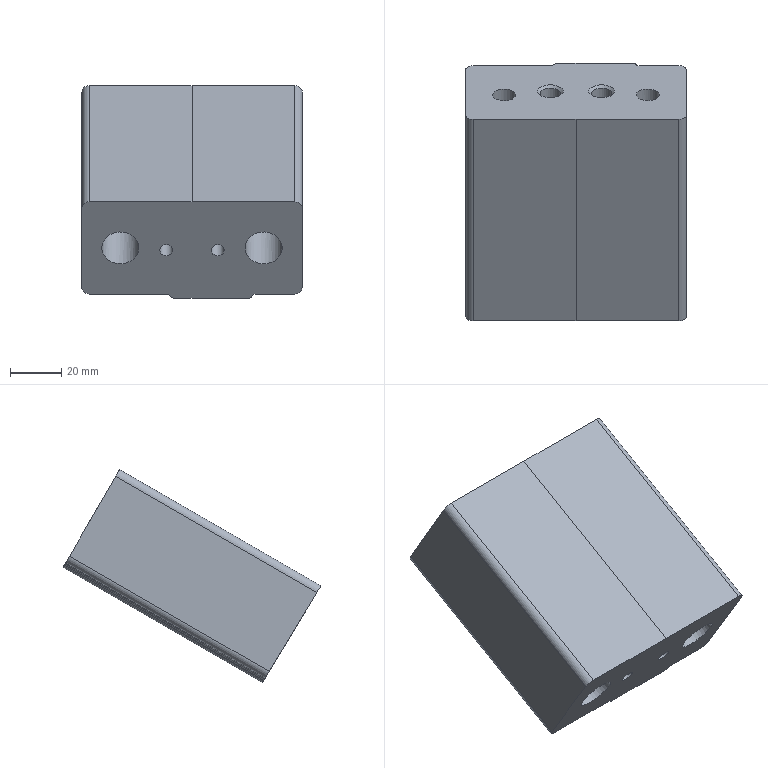Part | NX | features solid 2 | 1 solid | 32 faces | box 86.008 x 100.559 x 83.036 mm | volume 306507 mm3 | plane 13 | spline 9 | cylinder 8 | cone 2 | commonest cylinder face diameters 5.1 x2 8 x2 9.007 x2 14.508 x2
STEP:
#1=CARTESIAN_POINT('',(-139.757,107.914,-0.2414));
#2=VERTEX_POINT('',#1);
#3=CARTESIAN_POINT('',(-137.826,107.52,0.4097));
#4=CARTESIAN_POINT('',(-139.728,108.056,-0.4768));
#5=CARTESIAN_POINT('',(-141.803,107.738,0.04954));
#6=CARTESIAN_POINT('',(-142.834,106.756,1.674));
#7=CARTESIAN_POINT('',(-142.223,105.683,3.45));
#8=CARTESIAN_POINT('',(-140.322,105.148,4.335));
#9=CARTESIAN_POINT('',(-138.25,105.464,3.811));
#10=CARTESIAN_POINT('',(-137.215,106.447,2.186));
#11=CARTESIAN_POINT('',(-137.826,107.52,0.4097));
#12=CARTESIAN_POINT('',(-139.728,108.056,-0.4768));
#13=CARTESIAN_POINT('',(-141.803,107.738,0.04954));
#14=B_SPLINE_CURVE_WITH_KNOTS('',3,(#3,#4,#5,#6,#7,#8,#9,#10,#11,#12,#13),.UNSPECIFIED.,.T.,.F.,(1,1,1,1,1,1,1,1,1,1,1,1,1,1,1),(-0.005979,-0.003986,-0.001993,0.,0.001993,0.003986,0.005979,0.007972,0.009965,0.01196,0.01395,0.01594,0.01794,0.01993,0.02192),.UNSPECIFIED.);
#15=EDGE_CURVE('',#2,#2,#14,.T.);
#16=ORIENTED_EDGE('',*,*,#15,.T.);
#17=EDGE_LOOP('',(#16));
#18=FACE_BOUND('',#17,.T.);
#19=CARTESIAN_POINT('',(-170.771,106.072,2.807));
#20=VERTEX_POINT('',#19);
#21=CARTESIAN_POINT('',(-172.347,109.015,-2.062));
#22=CARTESIAN_POINT('',(-169.984,106.071,2.808));
#23=CARTESIAN_POINT('',(-172.341,103.131,7.673));
#24=CARTESIAN_POINT('',(-178.016,101.913,9.689));
#25=CARTESIAN_POINT('',(-183.705,103.128,7.681));
#26=CARTESIAN_POINT('',(-186.063,106.069,2.815));
#27=CARTESIAN_POINT('',(-183.717,109.007,-2.046));
#28=CARTESIAN_POINT('',(-178.037,110.229,-4.07));
#29=CARTESIAN_POINT('',(-172.347,109.015,-2.062));
#30=CARTESIAN_POINT('',(-169.984,106.071,2.808));
#31=CARTESIAN_POINT('',(-172.341,103.131,7.673));
#32=B_SPLINE_CURVE_WITH_KNOTS('',3,(#21,#22,#23,#24,#25,#26,#27,#28,#29,#30,#31),.UNSPECIFIED.,.T.,.F.,(1,1,1,1,1,1,1,1,1,1,1,1,1,1,1),(-0.01701,-0.01134,-0.005669,0.,0.005669,0.01134,0.01701,0.02268,0.02835,0.03402,0.03968,0.04535,0.05102,0.05669,0.06236),.UNSPECIFIED.);
#33=EDGE_CURVE('',#20,#20,#32,.T.);
#34=ORIENTED_EDGE('',*,*,#33,.F.);
#35=EDGE_LOOP('',(#34));
#36=FACE_BOUND('',#35,.T.);
#37=CARTESIAN_POINT('',(-129.279,106.076,2.8));
#38=VERTEX_POINT('',#37);
#39=CARTESIAN_POINT('',(-127.705,103.133,7.67));
#40=CARTESIAN_POINT('',(-130.066,106.077,2.798));
#41=CARTESIAN_POINT('',(-127.707,109.017,-2.066));
#42=CARTESIAN_POINT('',(-122.031,110.234,-4.079));
#43=CARTESIAN_POINT('',(-116.343,109.02,-2.068));
#44=CARTESIAN_POINT('',(-113.987,106.078,2.8));
#45=CARTESIAN_POINT('',(-116.335,103.141,7.659));
#46=CARTESIAN_POINT('',(-122.016,101.919,9.68));
#47=CARTESIAN_POINT('',(-127.705,103.133,7.67));
#48=CARTESIAN_POINT('',(-130.066,106.077,2.798));
#49=CARTESIAN_POINT('',(-127.707,109.017,-2.066));
#50=B_SPLINE_CURVE_WITH_KNOTS('',3,(#39,#40,#41,#42,#43,#44,#45,#46,#47,#48,#49),.UNSPECIFIED.,.T.,.F.,(1,1,1,1,1,1,1,1,1,1,1,1,1,1,1),(-0.01701,-0.01134,-0.005669,0.,0.005669,0.01134,0.01701,0.02268,0.02835,0.03402,0.03968,0.04535,0.05102,0.05669,0.06236),.UNSPECIFIED.);
#51=EDGE_CURVE('',#38,#38,#50,.T.);
#52=ORIENTED_EDGE('',*,*,#51,.F.);
#53=EDGE_LOOP('',(#52));
#54=FACE_BOUND('',#53,.T.);
#55=CARTESIAN_POINT('',(-110.021,95.216,20.774));
#56=VERTEX_POINT('',#55);
#57=CARTESIAN_POINT('',(-107.021,96.769,18.206));
#58=VERTEX_POINT('',#57);
#59=CARTESIAN_POINT('',(-110.021,95.216,20.774));
#60=CARTESIAN_POINT('',(-109.229,95.216,20.774));
#61=CARTESIAN_POINT('',(-107.676,95.554,20.216));
#62=CARTESIAN_POINT('',(-107.021,96.359,18.885));
#63=CARTESIAN_POINT('',(-107.021,96.769,18.206));
#64=B_SPLINE_CURVE_WITH_KNOTS('',3,(#59,#60,#61,#62,#63),.UNSPECIFIED.,.F.,.F.,(4,1,4),(0.,0.002343,0.004687),.UNSPECIFIED.);
#65=EDGE_CURVE('',#56,#58,#64,.T.);
#66=ORIENTED_EDGE('',*,*,#65,.F.);
#67=CARTESIAN_POINT('',(-150.023,95.214,20.773));
#68=VERTEX_POINT('',#67);
#69=CARTESIAN_POINT('',(-150.023,95.214,20.773));
#70=CARTESIAN_POINT('',(-136.689,95.213,20.773));
#71=CARTESIAN_POINT('',(-123.355,95.214,20.773));
#72=CARTESIAN_POINT('',(-110.021,95.216,20.774));
#73=B_SPLINE_CURVE_WITH_KNOTS('',3,(#69,#70,#71,#72),.UNSPECIFIED.,.F.,.F.,(4,4),(0.,0.04),.UNSPECIFIED.);
#74=EDGE_CURVE('',#68,#56,#73,.T.);
#75=ORIENTED_EDGE('',*,*,#74,.F.);
#76=CARTESIAN_POINT('',(-190.021,95.216,20.774));
#77=VERTEX_POINT('',#76);
#78=CARTESIAN_POINT('',(-190.021,95.216,20.774));
#79=CARTESIAN_POINT('',(-176.688,95.215,20.773));
#80=CARTESIAN_POINT('',(-163.356,95.214,20.773));
#81=CARTESIAN_POINT('',(-150.023,95.214,20.773));
#82=B_SPLINE_CURVE_WITH_KNOTS('',3,(#78,#79,#80,#81),.UNSPECIFIED.,.F.,.F.,(4,4),(0.,0.04),.UNSPECIFIED.);
#83=EDGE_CURVE('',#77,#68,#82,.T.);
#84=ORIENTED_EDGE('',*,*,#83,.F.);
#85=CARTESIAN_POINT('',(-193.021,96.768,18.208));
#86=VERTEX_POINT('',#85);
#87=CARTESIAN_POINT('',(-193.021,96.768,18.208));
#88=CARTESIAN_POINT('',(-193.021,96.358,18.886));
#89=CARTESIAN_POINT('',(-192.369,95.555,20.214));
#90=CARTESIAN_POINT('',(-190.813,95.216,20.774));
#91=CARTESIAN_POINT('',(-190.021,95.216,20.774));
#92=B_SPLINE_CURVE_WITH_KNOTS('',3,(#87,#88,#89,#90,#91),.UNSPECIFIED.,.F.,.F.,(4,1,4),(0.,0.002342,0.004684),.UNSPECIFIED.);
#93=EDGE_CURVE('',#86,#77,#92,.T.);
#94=ORIENTED_EDGE('',*,*,#93,.F.);
#95=CARTESIAN_POINT('',(-193.029,115.406,-12.632));
#96=VERTEX_POINT('',#95);
#97=CARTESIAN_POINT('',(-193.029,115.406,-12.632));
#98=CARTESIAN_POINT('',(-193.026,109.193,-2.352));
#99=CARTESIAN_POINT('',(-193.024,102.98,7.927));
#100=CARTESIAN_POINT('',(-193.021,96.768,18.208));
#101=B_SPLINE_CURVE_WITH_KNOTS('',3,(#97,#98,#99,#100),.UNSPECIFIED.,.F.,.F.,(4,4),(0.,0.03603),.UNSPECIFIED.);
#102=EDGE_CURVE('',#96,#86,#101,.T.);
#103=ORIENTED_EDGE('',*,*,#102,.F.);
#104=CARTESIAN_POINT('',(-190.029,116.958,-15.2));
#105=VERTEX_POINT('',#104);
#106=CARTESIAN_POINT('',(-190.029,116.958,-15.2));
#107=CARTESIAN_POINT('',(-190.821,116.958,-15.2));
#108=CARTESIAN_POINT('',(-192.374,116.621,-14.642));
#109=CARTESIAN_POINT('',(-193.029,115.816,-13.31));
#110=CARTESIAN_POINT('',(-193.029,115.406,-12.632));
#111=B_SPLINE_CURVE_WITH_KNOTS('',3,(#106,#107,#108,#109,#110),.UNSPECIFIED.,.F.,.F.,(4,1,4),(0.,0.002343,0.004687),.UNSPECIFIED.);
#112=EDGE_CURVE('',#105,#96,#111,.T.);
#113=ORIENTED_EDGE('',*,*,#112,.F.);
#114=CARTESIAN_POINT('',(-160.273,116.956,-15.202));
#115=VERTEX_POINT('',#114);
#116=CARTESIAN_POINT('',(-160.273,116.956,-15.202));
#117=CARTESIAN_POINT('',(-170.192,116.956,-15.202));
#118=CARTESIAN_POINT('',(-180.11,116.957,-15.201));
#119=CARTESIAN_POINT('',(-190.029,116.958,-15.2));
#120=B_SPLINE_CURVE_WITH_KNOTS('',3,(#116,#117,#118,#119),.UNSPECIFIED.,.F.,.F.,(4,4),(0.,0.02976),.UNSPECIFIED.);
#121=EDGE_CURVE('',#115,#105,#120,.T.);
#122=ORIENTED_EDGE('',*,*,#121,.F.);
#123=CARTESIAN_POINT('',(-158.541,117.473,-16.058));
#124=VERTEX_POINT('',#123);
#125=CARTESIAN_POINT('',(-158.541,117.473,-16.058));
#126=CARTESIAN_POINT('',(-158.893,117.158,-15.536));
#127=CARTESIAN_POINT('',(-159.57,116.956,-15.202));
#128=CARTESIAN_POINT('',(-160.273,116.956,-15.202));
#129=B_SPLINE_CURVE_WITH_KNOTS('',3,(#125,#126,#127,#128),.UNSPECIFIED.,.F.,.F.,(4,4),(0.,0.002093),.UNSPECIFIED.);
#130=EDGE_CURVE('',#124,#115,#129,.T.);
#131=ORIENTED_EDGE('',*,*,#130,.F.);
#132=CARTESIAN_POINT('',(-156.809,117.99,-16.913));
#133=VERTEX_POINT('',#132);
#134=CARTESIAN_POINT('',(-156.809,117.99,-16.913));
#135=CARTESIAN_POINT('',(-157.513,117.99,-16.913));
#136=CARTESIAN_POINT('',(-158.19,117.788,-16.579));
#137=CARTESIAN_POINT('',(-158.541,117.473,-16.058));
#138=B_SPLINE_CURVE_WITH_KNOTS('',3,(#134,#135,#136,#137),.UNSPECIFIED.,.F.,.F.,(4,4),(0.,0.002093),.UNSPECIFIED.);
#139=EDGE_CURVE('',#133,#124,#138,.T.);
#140=ORIENTED_EDGE('',*,*,#139,.F.);
#141=CARTESIAN_POINT('',(-150.023,117.99,-16.914));
#142=VERTEX_POINT('',#141);
#143=CARTESIAN_POINT('',(-150.023,117.99,-16.914));
#144=CARTESIAN_POINT('',(-152.285,117.99,-16.914));
#145=CARTESIAN_POINT('',(-154.547,117.99,-16.914));
#146=CARTESIAN_POINT('',(-156.809,117.99,-16.913));
#147=B_SPLINE_CURVE_WITH_KNOTS('',3,(#143,#144,#145,#146),.UNSPECIFIED.,.F.,.F.,(4,4),(0.,0.006786),.UNSPECIFIED.);
#148=EDGE_CURVE('',#142,#133,#147,.T.);
#149=ORIENTED_EDGE('',*,*,#148,.F.);
#150=CARTESIAN_POINT('',(-128.427,117.991,-16.913));
#151=VERTEX_POINT('',#150);
#152=CARTESIAN_POINT('',(-128.427,117.991,-16.913));
#153=CARTESIAN_POINT('',(-135.626,117.99,-16.913));
#154=CARTESIAN_POINT('',(-142.825,117.99,-16.914));
#155=CARTESIAN_POINT('',(-150.023,117.99,-16.914));
#156=B_SPLINE_CURVE_WITH_KNOTS('',3,(#152,#153,#154,#155),.UNSPECIFIED.,.F.,.F.,(4,4),(0.,0.0216),.UNSPECIFIED.);
#157=EDGE_CURVE('',#151,#142,#156,.T.);
#158=ORIENTED_EDGE('',*,*,#157,.F.);
#159=CARTESIAN_POINT('',(-126.695,117.474,-16.057));
#160=VERTEX_POINT('',#159);
#161=CARTESIAN_POINT('',(-126.695,117.474,-16.057));
#162=CARTESIAN_POINT('',(-127.047,117.789,-16.579));
#163=CARTESIAN_POINT('',(-127.724,117.991,-16.913));
#164=CARTESIAN_POINT('',(-128.427,117.991,-16.913));
#165=B_SPLINE_CURVE_WITH_KNOTS('',3,(#161,#162,#163,#164),.UNSPECIFIED.,.F.,.F.,(4,4),(0.,0.002093),.UNSPECIFIED.);
#166=EDGE_CURVE('',#160,#151,#165,.T.);
#167=ORIENTED_EDGE('',*,*,#166,.F.);
#168=CARTESIAN_POINT('',(-124.963,116.956,-15.201));
#169=VERTEX_POINT('',#168);
#170=CARTESIAN_POINT('',(-124.963,116.956,-15.201));
#171=CARTESIAN_POINT('',(-125.667,116.956,-15.201));
#172=CARTESIAN_POINT('',(-126.343,117.159,-15.536));
#173=CARTESIAN_POINT('',(-126.695,117.474,-16.057));
#174=B_SPLINE_CURVE_WITH_KNOTS('',3,(#170,#171,#172,#173),.UNSPECIFIED.,.F.,.F.,(4,4),(0.,0.002093),.UNSPECIFIED.);
#175=EDGE_CURVE('',#169,#160,#174,.T.);
#176=ORIENTED_EDGE('',*,*,#175,.F.);
#177=CARTESIAN_POINT('',(-110.029,116.958,-15.2));
#178=VERTEX_POINT('',#177);
#179=CARTESIAN_POINT('',(-110.029,116.958,-15.2));
#180=CARTESIAN_POINT('',(-115.007,116.957,-15.201));
#181=CARTESIAN_POINT('',(-119.985,116.957,-15.201));
#182=CARTESIAN_POINT('',(-124.963,116.956,-15.201));
#183=B_SPLINE_CURVE_WITH_KNOTS('',3,(#179,#180,#181,#182),.UNSPECIFIED.,.F.,.F.,(4,4),(0.,0.01493),.UNSPECIFIED.);
#184=EDGE_CURVE('',#178,#169,#183,.T.);
#185=ORIENTED_EDGE('',*,*,#184,.F.);
#186=CARTESIAN_POINT('',(-107.029,115.407,-12.633));
#187=VERTEX_POINT('',#186);
#188=CARTESIAN_POINT('',(-107.029,115.407,-12.633));
#189=CARTESIAN_POINT('',(-107.029,115.817,-13.311));
#190=CARTESIAN_POINT('',(-107.681,116.62,-14.64));
#191=CARTESIAN_POINT('',(-109.237,116.958,-15.2));
#192=CARTESIAN_POINT('',(-110.029,116.958,-15.2));
#193=B_SPLINE_CURVE_WITH_KNOTS('',3,(#188,#189,#190,#191,#192),.UNSPECIFIED.,.F.,.F.,(4,1,4),(0.,0.002343,0.004686),.UNSPECIFIED.);
#194=EDGE_CURVE('',#187,#178,#193,.T.);
#195=ORIENTED_EDGE('',*,*,#194,.F.);
#196=CARTESIAN_POINT('',(-107.021,96.769,18.206));
#197=CARTESIAN_POINT('',(-107.024,102.981,7.926));
#198=CARTESIAN_POINT('',(-107.026,109.194,-2.354));
#199=CARTESIAN_POINT('',(-107.029,115.407,-12.633));
#200=B_SPLINE_CURVE_WITH_KNOTS('',3,(#196,#197,#198,#199),.UNSPECIFIED.,.F.,.F.,(4,4),(0.,0.03603),.UNSPECIFIED.);
#201=EDGE_CURVE('',#58,#187,#200,.T.);
#202=ORIENTED_EDGE('',*,*,#201,.F.);
#203=EDGE_LOOP('',(#66,#75,#84,#94,#103,#113,#122,#131,#140,#149,#158,#167,#176,#185,#195,#202));
#204=FACE_BOUND('',#203,.T.);
#205=CARTESIAN_POINT('',(-159.757,107.914,-0.2413));
#206=VERTEX_POINT('',#205);
#207=CARTESIAN_POINT('',(-157.826,107.52,0.4098));
#208=CARTESIAN_POINT('',(-159.728,108.056,-0.4768));
#209=CARTESIAN_POINT('',(-161.803,107.738,0.0497));
#210=CARTESIAN_POINT('',(-162.834,106.756,1.674));
#211=CARTESIAN_POINT('',(-162.223,105.683,3.45));
#212=CARTESIAN_POINT('',(-160.322,105.148,4.335));
#213=CARTESIAN_POINT('',(-158.25,105.464,3.811));
#214=CARTESIAN_POINT('',(-157.215,106.447,2.186));
#215=CARTESIAN_POINT('',(-157.826,107.52,0.4098));
#216=CARTESIAN_POINT('',(-159.728,108.056,-0.4768));
#217=CARTESIAN_POINT('',(-161.803,107.738,0.0497));
#218=B_SPLINE_CURVE_WITH_KNOTS('',3,(#207,#208,#209,#210,#211,#212,#213,#214,#215,#216,#217),.UNSPECIFIED.,.T.,.F.,(1,1,1,1,1,1,1,1,1,1,1,1,1,1,1),(-0.005979,-0.003986,-0.001993,0.,0.001993,0.003986,0.005979,0.007972,0.009965,0.01196,0.01395,0.01594,0.01794,0.01993,0.02192),.UNSPECIFIED.);
#219=EDGE_CURVE('',#206,#206,#218,.T.);
#220=ORIENTED_EDGE('',*,*,#219,.T.);
#221=EDGE_LOOP('',(#220));
#222=FACE_BOUND('',#221,.T.);
#223=CARTESIAN_POINT('',(-193.54,95.075,21.009));
#224=CARTESIAN_POINT('',(-193.54,95.31,20.621));
#225=CARTESIAN_POINT('',(-193.542,102.949,7.979));
#226=CARTESIAN_POINT('',(-193.544,110.589,-4.661));
#227=CARTESIAN_POINT('',(-193.545,117.994,-16.913));
#228=CARTESIAN_POINT('',(-164.528,95.073,21.004));
#229=CARTESIAN_POINT('',(-164.528,95.308,20.615));
#230=CARTESIAN_POINT('',(-164.53,102.947,7.974));
#231=CARTESIAN_POINT('',(-164.532,110.587,-4.666));
#232=CARTESIAN_POINT('',(-164.534,117.992,-16.918));
#233=CARTESIAN_POINT('',(-135.516,95.074,21.));
#234=CARTESIAN_POINT('',(-135.517,95.309,20.612));
#235=CARTESIAN_POINT('',(-135.518,102.948,7.971));
#236=CARTESIAN_POINT('',(-135.52,110.588,-4.67));
#237=CARTESIAN_POINT('',(-135.522,117.993,-16.922));
#238=CARTESIAN_POINT('',(-106.505,95.08,21.));
#239=CARTESIAN_POINT('',(-106.505,95.315,20.612));
#240=CARTESIAN_POINT('',(-106.506,102.954,7.971));
#241=CARTESIAN_POINT('',(-106.508,110.594,-4.67));
#242=CARTESIAN_POINT('',(-106.51,117.999,-16.922));
#243=B_SPLINE_SURFACE_WITH_KNOTS('',3,3,((#223,#224,#225,#226,#227),(#228,#229,#230,#231,#232),(#233,#234,#235,#236,#237),(#238,#239,#240,#241,#242)),.UNSPECIFIED.,.F.,.F.,.F.,(4,4),(4,1,4),(0.02905,0.971),(-0.03172,0.,1.),.UNSPECIFIED.);
#244=ADVANCED_FACE('',(#18,#36,#54,#204,#222),#243,.F.);
#245=CARTESIAN_POINT('',(-107.029,193.273,32.325));
#246=VERTEX_POINT('',#245);
#247=CARTESIAN_POINT('',(-107.029,159.412,12.774));
#248=DIRECTION('',(0.000000832,0.866,0.5));
#249=VECTOR('',#248,1000.);
#250=LINE('',#247,#249);
#251=EDGE_CURVE('',#246,#187,#250,.F.);
#252=ORIENTED_EDGE('',*,*,#251,.T.);
#253=ORIENTED_EDGE('',*,*,#194,.T.);
#254=CARTESIAN_POINT('',(-110.029,194.773,29.728));
#255=VERTEX_POINT('',#254);
#256=CARTESIAN_POINT('',(-110.029,160.911,10.177));
#257=DIRECTION('',(0.000000832,0.866,0.5));
#258=VECTOR('',#257,1000.);
#259=LINE('',#256,#258);
#260=EDGE_CURVE('',#255,#178,#259,.F.);
#261=ORIENTED_EDGE('',*,*,#260,.F.);
#262=CARTESIAN_POINT('',(-107.029,193.273,32.325));
#263=CARTESIAN_POINT('',(-107.029,193.669,31.639));
#264=CARTESIAN_POINT('',(-107.681,194.445,30.294));
#265=CARTESIAN_POINT('',(-109.237,194.773,29.728));
#266=CARTESIAN_POINT('',(-110.029,194.773,29.728));
#267=B_SPLINE_CURVE_WITH_KNOTS('',3,(#262,#263,#264,#265,#266),.UNSPECIFIED.,.F.,.F.,(4,1,4),(0.,0.002343,0.004685),.UNSPECIFIED.);
#268=EDGE_CURVE('',#246,#255,#267,.T.);
#269=ORIENTED_EDGE('',*,*,#268,.F.);
#270=EDGE_LOOP('',(#252,#253,#261,#269));
#271=FACE_BOUND('',#270,.T.);
#272=CARTESIAN_POINT('',(-107.029,114.94,-12.903));
#273=CARTESIAN_POINT('',(-107.029,193.273,32.325));
#274=CARTESIAN_POINT('',(-107.029,115.332,-13.582));
#275=CARTESIAN_POINT('',(-107.029,193.666,31.645));
#276=CARTESIAN_POINT('',(-107.679,116.115,-14.939));
#277=CARTESIAN_POINT('',(-107.679,194.449,30.289));
#278=CARTESIAN_POINT('',(-109.247,116.439,-15.5));
#279=CARTESIAN_POINT('',(-109.247,194.773,29.728));
#280=CARTESIAN_POINT('',(-110.029,116.439,-15.5));
#281=CARTESIAN_POINT('',(-110.029,194.773,29.728));
#282=B_SPLINE_SURFACE_WITH_KNOTS('',3,1,((#272,#273),(#274,#275),(#276,#277),(#278,#279),(#280,#281)),.SURF_OF_LINEAR_EXTRUSION.,.F.,.F.,.F.,(4,1,4),(2,2),(0.,0.5,1.),(0.,1.),.UNSPECIFIED.);
#283=ADVANCED_FACE('',(#271),#282,.T.);
#284=ORIENTED_EDGE('',*,*,#260,.T.);
#285=ORIENTED_EDGE('',*,*,#184,.T.);
#286=CARTESIAN_POINT('',(-124.963,194.773,29.728));
#287=VERTEX_POINT('',#286);
#288=CARTESIAN_POINT('',(-124.963,160.911,10.177));
#289=DIRECTION('',(0.000000832,0.866,0.5));
#290=VECTOR('',#289,1000.);
#291=LINE('',#288,#290);
#292=EDGE_CURVE('',#287,#169,#291,.F.);
#293=ORIENTED_EDGE('',*,*,#292,.F.);
#294=CARTESIAN_POINT('',(-150.099,194.773,29.728));
#295=DIRECTION('',(1.,-0.000001199,0.000000412));
#296=VECTOR('',#295,1000.);
#297=LINE('',#294,#296);
#298=EDGE_CURVE('',#255,#287,#297,.F.);
#299=ORIENTED_EDGE('',*,*,#298,.F.);
#300=EDGE_LOOP('',(#284,#285,#293,#299));
#301=FACE_BOUND('',#300,.T.);
#302=CARTESIAN_POINT('',(-110.029,160.911,10.177));
#303=DIRECTION('',(0.000000956,0.5,-0.866));
#304=DIRECTION('',(-1.,0.000001199,-0.000000412));
#305=AXIS2_PLACEMENT_3D('',#302,#303,#304);
#306=PLANE('',#305);
#307=ADVANCED_FACE('',(#301),#306,.T.);
#308=ORIENTED_EDGE('',*,*,#292,.T.);
#309=ORIENTED_EDGE('',*,*,#175,.T.);
#310=CARTESIAN_POINT('',(-126.695,195.273,28.862));
#311=VERTEX_POINT('',#310);
#312=CARTESIAN_POINT('',(-126.695,161.411,9.311));
#313=DIRECTION('',(0.000000832,0.866,0.5));
#314=VECTOR('',#313,1000.);
#315=LINE('',#312,#314);
#316=EDGE_CURVE('',#311,#160,#315,.F.);
#317=ORIENTED_EDGE('',*,*,#316,.F.);
#318=CARTESIAN_POINT('',(-124.963,194.773,29.728));
#319=CARTESIAN_POINT('',(-125.666,194.773,29.728));
#320=CARTESIAN_POINT('',(-126.343,194.968,29.389));
#321=CARTESIAN_POINT('',(-126.695,195.273,28.862));
#322=B_SPLINE_CURVE_WITH_KNOTS('',3,(#318,#319,#320,#321),.UNSPECIFIED.,.F.,.F.,(4,4),(0.,0.002093),.UNSPECIFIED.);
#323=EDGE_CURVE('',#287,#311,#322,.T.);
#324=ORIENTED_EDGE('',*,*,#323,.F.);
#325=EDGE_LOOP('',(#308,#309,#317,#324));
#326=FACE_BOUND('',#325,.T.);
#327=CARTESIAN_POINT('',(-124.963,116.49,-15.471));
#328=CARTESIAN_POINT('',(-124.963,194.773,29.728));
#329=CARTESIAN_POINT('',(-125.661,116.49,-15.471));
#330=CARTESIAN_POINT('',(-125.661,194.773,29.728));
#331=CARTESIAN_POINT('',(-126.347,116.688,-15.815));
#332=CARTESIAN_POINT('',(-126.347,194.971,29.384));
#333=CARTESIAN_POINT('',(-126.695,116.989,-16.337));
#334=CARTESIAN_POINT('',(-126.695,195.273,28.862));
#335=B_SPLINE_SURFACE_WITH_KNOTS('',3,1,((#327,#328),(#329,#330),(#331,#332),(#333,#334)),.SURF_OF_LINEAR_EXTRUSION.,.F.,.F.,.F.,(4,4),(2,2),(0.,1.),(0.,1.),.PIECEWISE_BEZIER_KNOTS.);
#336=ADVANCED_FACE('',(#326),#335,.T.);
#337=ORIENTED_EDGE('',*,*,#316,.T.);
#338=ORIENTED_EDGE('',*,*,#166,.T.);
#339=CARTESIAN_POINT('',(-128.427,195.773,27.996));
#340=VERTEX_POINT('',#339);
#341=CARTESIAN_POINT('',(-128.427,161.911,8.445));
#342=DIRECTION('',(0.000000832,0.866,0.5));
#343=VECTOR('',#342,1000.);
#344=LINE('',#341,#343);
#345=EDGE_CURVE('',#340,#151,#344,.F.);
#346=ORIENTED_EDGE('',*,*,#345,.F.);
#347=CARTESIAN_POINT('',(-126.695,195.273,28.862));
#348=CARTESIAN_POINT('',(-127.047,195.577,28.334));
#349=CARTESIAN_POINT('',(-127.724,195.773,27.996));
#350=CARTESIAN_POINT('',(-128.427,195.773,27.996));
#351=B_SPLINE_CURVE_WITH_KNOTS('',3,(#347,#348,#349,#350),.UNSPECIFIED.,.F.,.F.,(4,4),(0.,0.002093),.UNSPECIFIED.);
#352=EDGE_CURVE('',#311,#340,#351,.T.);
#353=ORIENTED_EDGE('',*,*,#352,.F.);
#354=EDGE_LOOP('',(#337,#338,#346,#353));
#355=FACE_BOUND('',#354,.T.);
#356=CARTESIAN_POINT('',(-126.695,117.007,-16.327));
#357=CARTESIAN_POINT('',(-126.695,195.273,28.862));
#358=CARTESIAN_POINT('',(-127.044,117.309,-16.85));
#359=CARTESIAN_POINT('',(-127.044,195.575,28.339));
#360=CARTESIAN_POINT('',(-127.731,117.507,-17.193));
#361=CARTESIAN_POINT('',(-127.731,195.773,27.996));
#362=CARTESIAN_POINT('',(-128.427,117.507,-17.193));
#363=CARTESIAN_POINT('',(-128.427,195.773,27.996));
#364=B_SPLINE_SURFACE_WITH_KNOTS('',3,1,((#356,#357),(#358,#359),(#360,#361),(#362,#363)),.SURF_OF_LINEAR_EXTRUSION.,.F.,.F.,.F.,(4,4),(2,2),(0.,1.),(0.,1.),.PIECEWISE_BEZIER_KNOTS.);
#365=ADVANCED_FACE('',(#355),#364,.T.);
#366=ORIENTED_EDGE('',*,*,#345,.T.);
#367=ORIENTED_EDGE('',*,*,#157,.T.);
#368=CARTESIAN_POINT('',(-150.023,195.773,27.996));
#369=VERTEX_POINT('',#368);
#370=CARTESIAN_POINT('',(-150.023,161.911,8.445));
#371=DIRECTION('',(0.000000832,0.866,0.5));
#372=VECTOR('',#371,1000.);
#373=LINE('',#370,#372);
#374=EDGE_CURVE('',#369,#142,#373,.F.);
#375=ORIENTED_EDGE('',*,*,#374,.F.);
#376=CARTESIAN_POINT('',(-150.099,195.773,27.996));
#377=DIRECTION('',(1.,-0.000001199,0.000000412));
#378=VECTOR('',#377,1000.);
#379=LINE('',#376,#378);
#380=EDGE_CURVE('',#340,#369,#379,.F.);
#381=ORIENTED_EDGE('',*,*,#380,.F.);
#382=EDGE_LOOP('',(#366,#367,#375,#381));
#383=FACE_BOUND('',#382,.T.);
#384=CARTESIAN_POINT('',(-128.427,161.911,8.445));
#385=DIRECTION('',(0.000000956,0.5,-0.866));
#386=DIRECTION('',(-1.,0.000001199,-0.000000412));
#387=AXIS2_PLACEMENT_3D('',#384,#385,#386);
#388=PLANE('',#387);
#389=ADVANCED_FACE('',(#383),#388,.T.);
#390=ORIENTED_EDGE('',*,*,#374,.T.);
#391=ORIENTED_EDGE('',*,*,#148,.T.);
#392=CARTESIAN_POINT('',(-156.809,195.773,27.996));
#393=VERTEX_POINT('',#392);
#394=CARTESIAN_POINT('',(-156.809,161.911,8.445));
#395=DIRECTION('',(0.000000832,0.866,0.5));
#396=VECTOR('',#395,1000.);
#397=LINE('',#394,#396);
#398=EDGE_CURVE('',#393,#133,#397,.F.);
#399=ORIENTED_EDGE('',*,*,#398,.F.);
#400=CARTESIAN_POINT('',(-150.099,195.773,27.996));
#401=DIRECTION('',(1.,0.000001199,-0.000003741));
#402=VECTOR('',#401,1000.);
#403=LINE('',#400,#402);
#404=EDGE_CURVE('',#369,#393,#403,.F.);
#405=ORIENTED_EDGE('',*,*,#404,.F.);
#406=EDGE_LOOP('',(#390,#391,#399,#405));
#407=FACE_BOUND('',#406,.T.);
#408=CARTESIAN_POINT('',(-150.023,161.911,8.445));
#409=DIRECTION('',(-0.000003839,0.5,-0.866));
#410=DIRECTION('',(-1.,-0.000001199,0.000003741));
#411=AXIS2_PLACEMENT_3D('',#408,#409,#410);
#412=PLANE('',#411);
#413=ADVANCED_FACE('',(#407),#412,.T.);
#414=ORIENTED_EDGE('',*,*,#398,.T.);
#415=ORIENTED_EDGE('',*,*,#139,.T.);
#416=CARTESIAN_POINT('',(-158.541,195.273,28.862));
#417=VERTEX_POINT('',#416);
#418=CARTESIAN_POINT('',(-158.541,161.411,9.311));
#419=DIRECTION('',(0.000000832,0.866,0.5));
#420=VECTOR('',#419,1000.);
#421=LINE('',#418,#420);
#422=EDGE_CURVE('',#417,#124,#421,.F.);
#423=ORIENTED_EDGE('',*,*,#422,.F.);
#424=CARTESIAN_POINT('',(-156.809,195.773,27.996));
#425=CARTESIAN_POINT('',(-157.513,195.773,27.996));
#426=CARTESIAN_POINT('',(-158.19,195.577,28.334));
#427=CARTESIAN_POINT('',(-158.541,195.273,28.862));
#428=B_SPLINE_CURVE_WITH_KNOTS('',3,(#424,#425,#426,#427),.UNSPECIFIED.,.F.,.F.,(4,4),(0.,0.002093),.UNSPECIFIED.);
#429=EDGE_CURVE('',#393,#417,#428,.T.);
#430=ORIENTED_EDGE('',*,*,#429,.F.);
#431=EDGE_LOOP('',(#414,#415,#423,#430));
#432=FACE_BOUND('',#431,.T.);
#433=CARTESIAN_POINT('',(-156.809,117.506,-17.193));
#434=CARTESIAN_POINT('',(-156.809,195.773,27.996));
#435=CARTESIAN_POINT('',(-157.507,117.506,-17.193));
#436=CARTESIAN_POINT('',(-157.507,195.773,27.996));
#437=CARTESIAN_POINT('',(-158.193,117.307,-16.849));
#438=CARTESIAN_POINT('',(-158.193,195.574,28.34));
#439=CARTESIAN_POINT('',(-158.541,117.006,-16.327));
#440=CARTESIAN_POINT('',(-158.541,195.273,28.862));
#441=B_SPLINE_SURFACE_WITH_KNOTS('',3,1,((#433,#434),(#435,#436),(#437,#438),(#439,#440)),.SURF_OF_LINEAR_EXTRUSION.,.F.,.F.,.F.,(4,4),(2,2),(0.,1.),(0.,1.),.PIECEWISE_BEZIER_KNOTS.);
#442=ADVANCED_FACE('',(#432),#441,.T.);
#443=ORIENTED_EDGE('',*,*,#422,.T.);
#444=ORIENTED_EDGE('',*,*,#130,.T.);
#445=CARTESIAN_POINT('',(-160.273,194.773,29.728));
#446=VERTEX_POINT('',#445);
#447=CARTESIAN_POINT('',(-160.273,160.911,10.177));
#448=DIRECTION('',(0.000000832,0.866,0.5));
#449=VECTOR('',#448,1000.);
#450=LINE('',#447,#449);
#451=EDGE_CURVE('',#446,#115,#450,.F.);
#452=ORIENTED_EDGE('',*,*,#451,.F.);
#453=CARTESIAN_POINT('',(-158.541,195.273,28.862));
#454=CARTESIAN_POINT('',(-158.893,194.968,29.389));
#455=CARTESIAN_POINT('',(-159.57,194.773,29.728));
#456=CARTESIAN_POINT('',(-160.273,194.773,29.728));
#457=B_SPLINE_CURVE_WITH_KNOTS('',3,(#453,#454,#455,#456),.UNSPECIFIED.,.F.,.F.,(4,4),(0.,0.002093),.UNSPECIFIED.);
#458=EDGE_CURVE('',#417,#446,#457,.T.);
#459=ORIENTED_EDGE('',*,*,#458,.F.);
#460=EDGE_LOOP('',(#443,#444,#452,#459));
#461=FACE_BOUND('',#460,.T.);
#462=CARTESIAN_POINT('',(-158.541,116.989,-16.337));
#463=CARTESIAN_POINT('',(-158.541,195.273,28.862));
#464=CARTESIAN_POINT('',(-158.89,116.687,-15.814));
#465=CARTESIAN_POINT('',(-158.89,194.971,29.385));
#466=CARTESIAN_POINT('',(-159.578,116.489,-15.471));
#467=CARTESIAN_POINT('',(-159.578,194.773,29.728));
#468=CARTESIAN_POINT('',(-160.273,116.489,-15.471));
#469=CARTESIAN_POINT('',(-160.273,194.773,29.728));
#470=B_SPLINE_SURFACE_WITH_KNOTS('',3,1,((#462,#463),(#464,#465),(#466,#467),(#468,#469)),.SURF_OF_LINEAR_EXTRUSION.,.F.,.F.,.F.,(4,4),(2,2),(0.,1.),(0.,1.),.PIECEWISE_BEZIER_KNOTS.);
#471=ADVANCED_FACE('',(#461),#470,.T.);
#472=ORIENTED_EDGE('',*,*,#451,.T.);
#473=ORIENTED_EDGE('',*,*,#121,.T.);
#474=CARTESIAN_POINT('',(-190.029,194.773,29.728));
#475=VERTEX_POINT('',#474);
#476=CARTESIAN_POINT('',(-190.029,160.911,10.177));
#477=DIRECTION('',(0.000000832,0.866,0.5));
#478=VECTOR('',#477,1000.);
#479=LINE('',#476,#478);
#480=EDGE_CURVE('',#475,#105,#479,.F.);
#481=ORIENTED_EDGE('',*,*,#480,.F.);
#482=CARTESIAN_POINT('',(-150.099,194.773,29.728));
#483=DIRECTION('',(1.,0.000001199,-0.000003741));
#484=VECTOR('',#483,1000.);
#485=LINE('',#482,#484);
#486=EDGE_CURVE('',#446,#475,#485,.F.);
#487=ORIENTED_EDGE('',*,*,#486,.F.);
#488=EDGE_LOOP('',(#472,#473,#481,#487));
#489=FACE_BOUND('',#488,.T.);
#490=CARTESIAN_POINT('',(-160.273,160.911,10.177));
#491=DIRECTION('',(-0.000003839,0.5,-0.866));
#492=DIRECTION('',(-1.,-0.000001199,0.000003741));
#493=AXIS2_PLACEMENT_3D('',#490,#491,#492);
#494=PLANE('',#493);
#495=ADVANCED_FACE('',(#489),#494,.T.);
#496=ORIENTED_EDGE('',*,*,#480,.T.);
#497=ORIENTED_EDGE('',*,*,#112,.T.);
#498=CARTESIAN_POINT('',(-193.029,193.273,32.326));
#499=VERTEX_POINT('',#498);
#500=CARTESIAN_POINT('',(-193.029,159.411,12.775));
#501=DIRECTION('',(0.000000832,0.866,0.5));
#502=VECTOR('',#501,1000.);
#503=LINE('',#500,#502);
#504=EDGE_CURVE('',#499,#96,#503,.F.);
#505=ORIENTED_EDGE('',*,*,#504,.F.);
#506=CARTESIAN_POINT('',(-190.029,194.773,29.728));
#507=CARTESIAN_POINT('',(-190.821,194.773,29.728));
#508=CARTESIAN_POINT('',(-192.374,194.447,30.292));
#509=CARTESIAN_POINT('',(-193.029,193.669,31.64));
#510=CARTESIAN_POINT('',(-193.029,193.273,32.326));
#511=B_SPLINE_CURVE_WITH_KNOTS('',3,(#506,#507,#508,#509,#510),.UNSPECIFIED.,.F.,.F.,(4,1,4),(0.,0.002343,0.004686),.UNSPECIFIED.);
#512=EDGE_CURVE('',#475,#499,#511,.T.);
#513=ORIENTED_EDGE('',*,*,#512,.F.);
#514=EDGE_LOOP('',(#496,#497,#505,#513));
#515=FACE_BOUND('',#514,.T.);
#516=CARTESIAN_POINT('',(-190.029,116.439,-15.5));
#517=CARTESIAN_POINT('',(-190.029,194.773,29.728));
#518=CARTESIAN_POINT('',(-190.814,116.439,-15.5));
#519=CARTESIAN_POINT('',(-190.814,194.773,29.728));
#520=CARTESIAN_POINT('',(-192.381,116.115,-14.937));
#521=CARTESIAN_POINT('',(-192.38,194.448,30.29));
#522=CARTESIAN_POINT('',(-193.029,115.33,-13.579));
#523=CARTESIAN_POINT('',(-193.029,193.664,31.649));
#524=CARTESIAN_POINT('',(-193.029,114.939,-12.902));
#525=CARTESIAN_POINT('',(-193.029,193.273,32.326));
#526=B_SPLINE_SURFACE_WITH_KNOTS('',3,1,((#516,#517),(#518,#519),(#520,#521),(#522,#523),(#524,#525)),.SURF_OF_LINEAR_EXTRUSION.,.F.,.F.,.F.,(4,1,4),(2,2),(0.,0.5,1.),(0.,1.),.UNSPECIFIED.);
#527=ADVANCED_FACE('',(#515),#526,.T.);
#528=ORIENTED_EDGE('',*,*,#504,.T.);
#529=ORIENTED_EDGE('',*,*,#102,.T.);
#530=CARTESIAN_POINT('',(-193.021,175.259,63.526));
#531=VERTEX_POINT('',#530);
#532=CARTESIAN_POINT('',(-193.021,141.397,43.975));
#533=DIRECTION('',(0.000000832,0.866,0.5));
#534=VECTOR('',#533,1000.);
#535=LINE('',#532,#534);
#536=EDGE_CURVE('',#531,#86,#535,.F.);
#537=ORIENTED_EDGE('',*,*,#536,.F.);
#538=CARTESIAN_POINT('',(-193.025,185.26,46.203));
#539=DIRECTION('',(-0.0002148,0.5,-0.866));
#540=VECTOR('',#539,1000.);
#541=LINE('',#538,#540);
#542=EDGE_CURVE('',#499,#531,#541,.F.);
#543=ORIENTED_EDGE('',*,*,#542,.F.);
#544=EDGE_LOOP('',(#528,#529,#537,#543));
#545=FACE_BOUND('',#544,.T.);
#546=CARTESIAN_POINT('',(-193.029,159.411,12.775));
#547=DIRECTION('',(-1.,-0.0001067,0.0001864));
#548=DIRECTION('',(0.0002148,-0.5,0.866));
#549=AXIS2_PLACEMENT_3D('',#546,#547,#548);
#550=PLANE('',#549);
#551=ADVANCED_FACE('',(#545),#550,.T.);
#552=ORIENTED_EDGE('',*,*,#536,.T.);
#553=ORIENTED_EDGE('',*,*,#93,.T.);
#554=CARTESIAN_POINT('',(-190.021,173.759,66.123));
#555=VERTEX_POINT('',#554);
#556=CARTESIAN_POINT('',(-190.021,139.898,46.572));
#557=DIRECTION('',(0.000000832,0.866,0.5));
#558=VECTOR('',#557,1000.);
#559=LINE('',#556,#558);
#560=EDGE_CURVE('',#555,#77,#559,.F.);
#561=ORIENTED_EDGE('',*,*,#560,.F.);
#562=CARTESIAN_POINT('',(-193.021,175.259,63.526));
#563=CARTESIAN_POINT('',(-193.021,174.863,64.212));
#564=CARTESIAN_POINT('',(-192.368,174.086,65.556));
#565=CARTESIAN_POINT('',(-190.813,173.759,66.123));
#566=CARTESIAN_POINT('',(-190.021,173.759,66.123));
#567=B_SPLINE_CURVE_WITH_KNOTS('',3,(#562,#563,#564,#565,#566),.UNSPECIFIED.,.F.,.F.,(4,1,4),(0.,0.002342,0.004683),.UNSPECIFIED.);
#568=EDGE_CURVE('',#531,#555,#567,.T.);
#569=ORIENTED_EDGE('',*,*,#568,.F.);
#570=EDGE_LOOP('',(#552,#553,#561,#569));
#571=FACE_BOUND('',#570,.T.);
#572=CARTESIAN_POINT('',(-193.021,96.244,17.905));
#573=CARTESIAN_POINT('',(-193.021,175.259,63.526));
#574=CARTESIAN_POINT('',(-193.021,95.848,18.591));
#575=CARTESIAN_POINT('',(-193.021,174.863,64.212));
#576=CARTESIAN_POINT('',(-192.369,95.072,19.935));
#577=CARTESIAN_POINT('',(-192.368,174.086,65.556));
#578=CARTESIAN_POINT('',(-190.813,94.745,20.502));
#579=CARTESIAN_POINT('',(-190.813,173.759,66.123));
#580=CARTESIAN_POINT('',(-190.021,94.745,20.502));
#581=CARTESIAN_POINT('',(-190.021,173.759,66.123));
#582=B_SPLINE_SURFACE_WITH_KNOTS('',3,1,((#572,#573),(#574,#575),(#576,#577),(#578,#579),(#580,#581)),.SURF_OF_LINEAR_EXTRUSION.,.F.,.F.,.F.,(4,1,4),(2,2),(0.,0.5,1.),(0.,1.),.UNSPECIFIED.);
#583=ADVANCED_FACE('',(#571),#582,.T.);
#584=ORIENTED_EDGE('',*,*,#560,.T.);
#585=ORIENTED_EDGE('',*,*,#83,.T.);
#586=CARTESIAN_POINT('',(-150.023,173.759,66.123));
#587=VERTEX_POINT('',#586);
#588=CARTESIAN_POINT('',(-150.023,139.898,46.572));
#589=DIRECTION('',(0.000000832,0.866,0.5));
#590=VECTOR('',#589,1000.);
#591=LINE('',#588,#590);
#592=EDGE_CURVE('',#587,#68,#591,.F.);
#593=ORIENTED_EDGE('',*,*,#592,.F.);
#594=CARTESIAN_POINT('',(-150.099,173.759,66.123));
#595=DIRECTION('',(-1.,-0.000001199,0.000003741));
#596=VECTOR('',#595,1000.);
#597=LINE('',#594,#596);
#598=EDGE_CURVE('',#555,#587,#597,.F.);
#599=ORIENTED_EDGE('',*,*,#598,.F.);
#600=EDGE_LOOP('',(#584,#585,#593,#599));
#601=FACE_BOUND('',#600,.T.);
#602=CARTESIAN_POINT('',(-190.021,139.898,46.572));
#603=DIRECTION('',(0.000003839,-0.5,0.866));
#604=DIRECTION('',(1.,0.000001199,-0.000003741));
#605=AXIS2_PLACEMENT_3D('',#602,#603,#604);
#606=PLANE('',#605);
#607=ADVANCED_FACE('',(#601),#606,.T.);
#608=ORIENTED_EDGE('',*,*,#592,.T.);
#609=ORIENTED_EDGE('',*,*,#74,.T.);
#610=CARTESIAN_POINT('',(-110.021,173.759,66.123));
#611=VERTEX_POINT('',#610);
#612=CARTESIAN_POINT('',(-110.021,139.898,46.572));
#613=DIRECTION('',(0.000000832,0.866,0.5));
#614=VECTOR('',#613,1000.);
#615=LINE('',#612,#614);
#616=EDGE_CURVE('',#611,#56,#615,.F.);
#617=ORIENTED_EDGE('',*,*,#616,.F.);
#618=CARTESIAN_POINT('',(-150.099,173.759,66.123));
#619=DIRECTION('',(-1.,0.000001199,-0.000000412));
#620=VECTOR('',#619,1000.);
#621=LINE('',#618,#620);
#622=EDGE_CURVE('',#587,#611,#621,.F.);
#623=ORIENTED_EDGE('',*,*,#622,.F.);
#624=EDGE_LOOP('',(#608,#609,#617,#623));
#625=FACE_BOUND('',#624,.T.);
#626=CARTESIAN_POINT('',(-150.023,139.898,46.572));
#627=DIRECTION('',(-0.000000956,-0.5,0.866));
#628=DIRECTION('',(1.,-0.000001199,0.000000412));
#629=AXIS2_PLACEMENT_3D('',#626,#627,#628);
#630=PLANE('',#629);
#631=ADVANCED_FACE('',(#625),#630,.T.);
#632=ORIENTED_EDGE('',*,*,#616,.T.);
#633=ORIENTED_EDGE('',*,*,#65,.T.);
#634=CARTESIAN_POINT('',(-107.021,175.259,63.525));
#635=VERTEX_POINT('',#634);
#636=CARTESIAN_POINT('',(-107.021,141.398,43.974));
#637=DIRECTION('',(0.000000832,0.866,0.5));
#638=VECTOR('',#637,1000.);
#639=LINE('',#636,#638);
#640=EDGE_CURVE('',#635,#58,#639,.F.);
#641=ORIENTED_EDGE('',*,*,#640,.F.);
#642=CARTESIAN_POINT('',(-110.021,173.759,66.123));
#643=CARTESIAN_POINT('',(-109.229,173.759,66.123));
#644=CARTESIAN_POINT('',(-107.676,174.085,65.558));
#645=CARTESIAN_POINT('',(-107.021,174.863,64.211));
#646=CARTESIAN_POINT('',(-107.021,175.259,63.525));
#647=B_SPLINE_CURVE_WITH_KNOTS('',3,(#642,#643,#644,#645,#646),.UNSPECIFIED.,.F.,.F.,(4,1,4),(0.,0.002343,0.004686),.UNSPECIFIED.);
#648=EDGE_CURVE('',#611,#635,#647,.T.);
#649=ORIENTED_EDGE('',*,*,#648,.F.);
#650=EDGE_LOOP('',(#632,#633,#641,#649));
#651=FACE_BOUND('',#650,.T.);
#652=CARTESIAN_POINT('',(-110.021,94.745,20.502));
#653=CARTESIAN_POINT('',(-110.021,173.759,66.123));
#654=CARTESIAN_POINT('',(-109.236,94.745,20.502));
#655=CARTESIAN_POINT('',(-109.236,173.759,66.123));
#656=CARTESIAN_POINT('',(-107.669,95.07,19.94));
#657=CARTESIAN_POINT('',(-107.669,174.084,65.56));
#658=CARTESIAN_POINT('',(-107.021,95.854,18.581));
#659=CARTESIAN_POINT('',(-107.021,174.868,64.202));
#660=CARTESIAN_POINT('',(-107.021,96.245,17.904));
#661=CARTESIAN_POINT('',(-107.021,175.259,63.525));
#662=B_SPLINE_SURFACE_WITH_KNOTS('',3,1,((#652,#653),(#654,#655),(#656,#657),(#658,#659),(#660,#661)),.SURF_OF_LINEAR_EXTRUSION.,.F.,.F.,.F.,(4,1,4),(2,2),(0.,0.5,1.),(0.,1.),.UNSPECIFIED.);
#663=ADVANCED_FACE('',(#651),#662,.T.);
#664=CARTESIAN_POINT('',(-107.025,185.27,46.187));
#665=DIRECTION('',(0.0002148,-0.5,0.866));
#666=VECTOR('',#665,1000.);
#667=LINE('',#664,#666);
#668=EDGE_CURVE('',#635,#246,#667,.F.);
#669=ORIENTED_EDGE('',*,*,#668,.F.);
#670=ORIENTED_EDGE('',*,*,#640,.T.);
#671=ORIENTED_EDGE('',*,*,#201,.T.);
#672=ORIENTED_EDGE('',*,*,#251,.F.);
#673=EDGE_LOOP('',(#669,#670,#671,#672));
#674=FACE_BOUND('',#673,.T.);
#675=CARTESIAN_POINT('',(-107.021,141.398,43.974));
#676=DIRECTION('',(1.,0.0001067,-0.0001864));
#677=DIRECTION('',(-0.0002148,0.5,-0.866));
#678=AXIS2_PLACEMENT_3D('',#675,#676,#677);
#679=PLANE('',#678);
#680=ADVANCED_FACE('',(#674),#679,.T.);
#681=CARTESIAN_POINT('',(-140.025,187.266,42.729));
#682=VERTEX_POINT('',#681);
#683=CARTESIAN_POINT('',(-140.025,184.766,47.059));
#684=DIRECTION('',(-0.000000832,-0.866,-0.5));
#685=DIRECTION('',(0.,0.5,-0.866));
#686=AXIS2_PLACEMENT_3D('',#683,#684,#685);
#687=CIRCLE('',#686,5.);
#688=EDGE_CURVE('',#682,#682,#687,.T.);
#689=ORIENTED_EDGE('',*,*,#688,.T.);
#690=EDGE_LOOP('',(#689));
#691=FACE_BOUND('',#690,.T.);
#692=CARTESIAN_POINT('',(-160.025,187.266,42.729));
#693=VERTEX_POINT('',#692);
#694=CARTESIAN_POINT('',(-160.025,184.766,47.059));
#695=DIRECTION('',(-0.000000832,-0.866,-0.5));
#696=DIRECTION('',(0.,0.5,-0.866));
#697=AXIS2_PLACEMENT_3D('',#694,#695,#696);
#698=CIRCLE('',#697,5.);
#699=EDGE_CURVE('',#693,#693,#698,.T.);
#700=ORIENTED_EDGE('',*,*,#699,.T.);
#701=EDGE_LOOP('',(#700));
#702=FACE_BOUND('',#701,.T.);
#703=CARTESIAN_POINT('',(-178.024,181.096,53.415));
#704=VERTEX_POINT('',#703);
#705=CARTESIAN_POINT('',(-178.025,183.348,49.515));
#706=DIRECTION('',(-0.000000832,-0.866,-0.5));
#707=DIRECTION('',(0.0001031,-0.5,0.866));
#708=AXIS2_PLACEMENT_3D('',#705,#706,#707);
#709=ELLIPSE('',#708,4.504,4.503);
#710=EDGE_CURVE('',#704,#704,#709,.T.);
#711=ORIENTED_EDGE('',*,*,#710,.T.);
#712=EDGE_LOOP('',(#711));
#713=FACE_BOUND('',#712,.T.);
#714=CARTESIAN_POINT('',(-122.023,181.102,53.405));
#715=VERTEX_POINT('',#714);
#716=CARTESIAN_POINT('',(-122.024,183.354,49.504));
#717=DIRECTION('',(-0.000000832,-0.866,-0.5));
#718=DIRECTION('',(0.0003265,-0.5,0.866));
#719=AXIS2_PLACEMENT_3D('',#716,#717,#718);
#720=ELLIPSE('',#719,4.504,4.503);
#721=EDGE_CURVE('',#715,#715,#720,.T.);
#722=ORIENTED_EDGE('',*,*,#721,.T.);
#723=EDGE_LOOP('',(#722));
#724=FACE_BOUND('',#723,.T.);
#725=ORIENTED_EDGE('',*,*,#648,.T.);
#726=ORIENTED_EDGE('',*,*,#668,.T.);
#727=ORIENTED_EDGE('',*,*,#268,.T.);
#728=ORIENTED_EDGE('',*,*,#298,.T.);
#729=ORIENTED_EDGE('',*,*,#323,.T.);
#730=ORIENTED_EDGE('',*,*,#352,.T.);
#731=ORIENTED_EDGE('',*,*,#380,.T.);
#732=ORIENTED_EDGE('',*,*,#404,.T.);
#733=ORIENTED_EDGE('',*,*,#429,.T.);
#734=ORIENTED_EDGE('',*,*,#458,.T.);
#735=ORIENTED_EDGE('',*,*,#486,.T.);
#736=ORIENTED_EDGE('',*,*,#512,.T.);
#737=ORIENTED_EDGE('',*,*,#542,.T.);
#738=ORIENTED_EDGE('',*,*,#568,.T.);
#739=ORIENTED_EDGE('',*,*,#598,.T.);
#740=ORIENTED_EDGE('',*,*,#622,.T.);
#741=EDGE_LOOP('',(#725,#726,#727,#728,#729,#730,#731,#732,#733,#734,#735,#736,#737,#738,#739,#740));
#742=FACE_BOUND('',#741,.T.);
#743=CARTESIAN_POINT('',(-150.099,185.265,46.195));
#744=DIRECTION('',(-0.000000832,-0.866,-0.5));
#745=DIRECTION('',(0.000001441,-0.5,0.866));
#746=AXIS2_PLACEMENT_3D('',#743,#744,#745);
#747=PLANE('',#746);
#748=ADVANCED_FACE('',(#691,#702,#713,#724,#742),#747,.F.);
#749=CARTESIAN_POINT('',(-178.025,134.933,14.992));
#750=VERTEX_POINT('',#749);
#751=CARTESIAN_POINT('',(-178.025,132.604,18.846));
#752=DIRECTION('',(0.000002895,0.8558,0.5172));
#753=DIRECTION('',(0.,0.5172,-0.8558));
#754=AXIS2_PLACEMENT_3D('',#751,#752,#753);
#755=CIRCLE('',#754,4.503);
#756=EDGE_CURVE('',#750,#750,#755,.F.);
#757=ORIENTED_EDGE('',*,*,#756,.T.);
#758=EDGE_LOOP('',(#757));
#759=FACE_BOUND('',#758,.T.);
#760=ORIENTED_EDGE('',*,*,#710,.F.);
#761=EDGE_LOOP('',(#760));
#762=FACE_BOUND('',#761,.T.);
#763=CARTESIAN_POINT('',(-178.025,106.073,2.811));
#764=DIRECTION('',(0.000002895,0.8558,0.5172));
#765=DIRECTION('',(1.,0.0002175,-0.0003655));
#766=AXIS2_PLACEMENT_3D('',#763,#764,#765);
#767=CYLINDRICAL_SURFACE('',#766,4.503);
#768=ADVANCED_FACE('',(#759,#762),#767,.F.);
#769=ORIENTED_EDGE('',*,*,#756,.F.);
#770=EDGE_LOOP('',(#769));
#771=FACE_BOUND('',#770,.T.);
#772=CARTESIAN_POINT('',(-178.025,136.356,12.638));
#773=VERTEX_POINT('',#772);
#774=CARTESIAN_POINT('',(-178.025,132.604,18.846));
#775=DIRECTION('',(0.000002895,0.8558,0.5172));
#776=DIRECTION('',(0.,0.5172,-0.8558));
#777=AXIS2_PLACEMENT_3D('',#774,#775,#776);
#778=CIRCLE('',#777,7.254);
#779=EDGE_CURVE('',#773,#773,#778,.F.);
#780=ORIENTED_EDGE('',*,*,#779,.T.);
#781=EDGE_LOOP('',(#780));
#782=FACE_BOUND('',#781,.T.);
#783=CARTESIAN_POINT('',(-178.025,132.604,18.846));
#784=DIRECTION('',(0.000002895,0.8558,0.5172));
#785=DIRECTION('',(-0.0004295,0.5172,-0.8558));
#786=AXIS2_PLACEMENT_3D('',#783,#784,#785);
#787=PLANE('',#786);
#788=ADVANCED_FACE('',(#771,#782),#787,.F.);
#789=ORIENTED_EDGE('',*,*,#779,.F.);
#790=EDGE_LOOP('',(#789));
#791=FACE_BOUND('',#790,.T.);
#792=ORIENTED_EDGE('',*,*,#33,.T.);
#793=EDGE_LOOP('',(#792));
#794=FACE_BOUND('',#793,.T.);
#795=CARTESIAN_POINT('',(-178.025,106.073,2.811));
#796=DIRECTION('',(0.000002895,0.8558,0.5172));
#797=DIRECTION('',(1.,0.0002175,-0.0003655));
#798=AXIS2_PLACEMENT_3D('',#795,#796,#797);
#799=CYLINDRICAL_SURFACE('',#798,7.254);
#800=ADVANCED_FACE('',(#791,#794),#799,.F.);
#801=CARTESIAN_POINT('',(-122.025,134.939,14.981));
#802=VERTEX_POINT('',#801);
#803=CARTESIAN_POINT('',(-122.025,132.61,18.836));
#804=DIRECTION('',(0.000007365,0.8558,0.5172));
#805=DIRECTION('',(0.,0.5172,-0.8558));
#806=AXIS2_PLACEMENT_3D('',#803,#804,#805);
#807=CIRCLE('',#806,4.503);
#808=EDGE_CURVE('',#802,#802,#807,.T.);
#809=ORIENTED_EDGE('',*,*,#808,.F.);
#810=EDGE_LOOP('',(#809));
#811=FACE_BOUND('',#810,.T.);
#812=ORIENTED_EDGE('',*,*,#721,.F.);
#813=EDGE_LOOP('',(#812));
#814=FACE_BOUND('',#813,.T.);
#815=CARTESIAN_POINT('',(-122.025,106.079,2.801));
#816=DIRECTION('',(0.000007365,0.8558,0.5172));
#817=DIRECTION('',(-1.,0.000004154,0.000007365));
#818=AXIS2_PLACEMENT_3D('',#815,#816,#817);
#819=CYLINDRICAL_SURFACE('',#818,4.503);
#820=ADVANCED_FACE('',(#811,#814),#819,.F.);
#821=ORIENTED_EDGE('',*,*,#808,.T.);
#822=EDGE_LOOP('',(#821));
#823=FACE_BOUND('',#822,.T.);
#824=CARTESIAN_POINT('',(-129.279,132.61,18.836));
#825=VERTEX_POINT('',#824);
#826=CARTESIAN_POINT('',(-122.025,132.61,18.836));
#827=DIRECTION('',(-0.000007365,-0.8558,-0.5172));
#828=DIRECTION('',(-1.,0.000004154,0.000007365));
#829=AXIS2_PLACEMENT_3D('',#826,#827,#828);
#830=CIRCLE('',#829,7.254);
#831=EDGE_CURVE('',#825,#825,#830,.F.);
#832=ORIENTED_EDGE('',*,*,#831,.F.);
#833=EDGE_LOOP('',(#832));
#834=FACE_BOUND('',#833,.T.);
#835=CARTESIAN_POINT('',(-122.025,132.61,18.836));
#836=DIRECTION('',(0.000007365,0.8558,0.5172));
#837=DIRECTION('',(0.,0.5172,-0.8558));
#838=AXIS2_PLACEMENT_3D('',#835,#836,#837);
#839=PLANE('',#838);
#840=ADVANCED_FACE('',(#823,#834),#839,.F.);
#841=ORIENTED_EDGE('',*,*,#831,.T.);
#842=EDGE_LOOP('',(#841));
#843=FACE_BOUND('',#842,.T.);
#844=ORIENTED_EDGE('',*,*,#51,.T.);
#845=EDGE_LOOP('',(#844));
#846=FACE_BOUND('',#845,.T.);
#847=CARTESIAN_POINT('',(-122.025,106.079,2.801));
#848=DIRECTION('',(0.000007365,0.8558,0.5172));
#849=DIRECTION('',(-1.,0.000004154,0.000007365));
#850=AXIS2_PLACEMENT_3D('',#847,#848,#849);
#851=CYLINDRICAL_SURFACE('',#850,7.254);
#852=ADVANCED_FACE('',(#843,#846),#851,.F.);
#853=CARTESIAN_POINT('',(-140.025,185.9,43.095));
#854=VERTEX_POINT('',#853);
#855=CARTESIAN_POINT('',(-140.025,183.9,46.559));
#856=DIRECTION('',(-0.000000832,-0.866,-0.5));
#857=DIRECTION('',(0.,0.5,-0.866));
#858=AXIS2_PLACEMENT_3D('',#855,#856,#857);
#859=CIRCLE('',#858,4.);
#860=EDGE_CURVE('',#854,#854,#859,.F.);
#861=ORIENTED_EDGE('',*,*,#860,.T.);
#862=EDGE_LOOP('',(#861));
#863=FACE_BOUND('',#862,.T.);
#864=CARTESIAN_POINT('',(-144.025,137.21,19.602));
#865=VERTEX_POINT('',#864);
#866=CARTESIAN_POINT('',(-140.025,137.21,19.602));
#867=DIRECTION('',(0.000000832,0.866,0.5));
#868=DIRECTION('',(-1.,0.,0.000001664));
#869=AXIS2_PLACEMENT_3D('',#866,#867,#868);
#870=CIRCLE('',#869,4.);
#871=EDGE_CURVE('',#865,#865,#870,.T.);
#872=ORIENTED_EDGE('',*,*,#871,.F.);
#873=EDGE_LOOP('',(#872));
#874=FACE_BOUND('',#873,.T.);
#875=CARTESIAN_POINT('',(-140.025,223.812,69.603));
#876=DIRECTION('',(-0.000000832,-0.866,-0.5));
#877=DIRECTION('',(0.,0.5,-0.866));
#878=AXIS2_PLACEMENT_3D('',#875,#876,#877);
#879=CYLINDRICAL_SURFACE('',#878,4.);
#880=ADVANCED_FACE('',(#863,#874),#879,.F.);
#881=ORIENTED_EDGE('',*,*,#15,.F.);
#882=EDGE_LOOP('',(#881));
#883=FACE_BOUND('',#882,.T.);
#884=CARTESIAN_POINT('',(-140.025,138.485,17.394));
#885=VERTEX_POINT('',#884);
#886=CARTESIAN_POINT('',(-140.025,137.21,19.602));
#887=DIRECTION('',(-0.000000832,-0.866,-0.5));
#888=DIRECTION('',(0.,0.5,-0.866));
#889=AXIS2_PLACEMENT_3D('',#886,#887,#888);
#890=CIRCLE('',#889,2.55);
#891=EDGE_CURVE('',#885,#885,#890,.F.);
#892=ORIENTED_EDGE('',*,*,#891,.T.);
#893=EDGE_LOOP('',(#892));
#894=FACE_BOUND('',#893,.T.);
#895=CARTESIAN_POINT('',(-140.025,106.034,1.602));
#896=DIRECTION('',(0.000000832,0.866,0.5));
#897=DIRECTION('',(0.,-0.5,0.866));
#898=AXIS2_PLACEMENT_3D('',#895,#896,#897);
#899=CYLINDRICAL_SURFACE('',#898,2.55);
#900=ADVANCED_FACE('',(#883,#894),#899,.F.);
#901=ORIENTED_EDGE('',*,*,#871,.T.);
#902=EDGE_LOOP('',(#901));
#903=FACE_BOUND('',#902,.T.);
#904=ORIENTED_EDGE('',*,*,#891,.F.);
#905=EDGE_LOOP('',(#904));
#906=FACE_BOUND('',#905,.T.);
#907=CARTESIAN_POINT('',(-140.025,137.21,19.602));
#908=DIRECTION('',(-0.000000832,-0.866,-0.5));
#909=DIRECTION('',(0.,0.5,-0.866));
#910=AXIS2_PLACEMENT_3D('',#907,#908,#909);
#911=PLANE('',#910);
#912=ADVANCED_FACE('',(#903,#906),#911,.F.);
#913=CARTESIAN_POINT('',(-160.025,185.9,43.095));
#914=VERTEX_POINT('',#913);
#915=CARTESIAN_POINT('',(-160.025,183.9,46.559));
#916=DIRECTION('',(-0.000000832,-0.866,-0.5));
#917=DIRECTION('',(0.,0.5,-0.866));
#918=AXIS2_PLACEMENT_3D('',#915,#916,#917);
#919=CIRCLE('',#918,4.);
#920=EDGE_CURVE('',#914,#914,#919,.F.);
#921=ORIENTED_EDGE('',*,*,#920,.T.);
#922=EDGE_LOOP('',(#921));
#923=FACE_BOUND('',#922,.T.);
#924=CARTESIAN_POINT('',(-164.025,137.21,19.602));
#925=VERTEX_POINT('',#924);
#926=CARTESIAN_POINT('',(-160.025,137.21,19.602));
#927=DIRECTION('',(0.000000832,0.866,0.5));
#928=DIRECTION('',(-1.,0.,0.000001664));
#929=AXIS2_PLACEMENT_3D('',#926,#927,#928);
#930=CIRCLE('',#929,4.);
#931=EDGE_CURVE('',#925,#925,#930,.T.);
#932=ORIENTED_EDGE('',*,*,#931,.F.);
#933=EDGE_LOOP('',(#932));
#934=FACE_BOUND('',#933,.T.);
#935=CARTESIAN_POINT('',(-160.025,223.812,69.603));
#936=DIRECTION('',(-0.000000832,-0.866,-0.5));
#937=DIRECTION('',(0.,0.5,-0.866));
#938=AXIS2_PLACEMENT_3D('',#935,#936,#937);
#939=CYLINDRICAL_SURFACE('',#938,4.);
#940=ADVANCED_FACE('',(#923,#934),#939,.F.);
#941=ORIENTED_EDGE('',*,*,#219,.F.);
#942=EDGE_LOOP('',(#941));
#943=FACE_BOUND('',#942,.T.);
#944=CARTESIAN_POINT('',(-160.025,138.485,17.394));
#945=VERTEX_POINT('',#944);
#946=CARTESIAN_POINT('',(-160.025,137.21,19.602));
#947=DIRECTION('',(-0.000000832,-0.866,-0.5));
#948=DIRECTION('',(0.,0.5,-0.866));
#949=AXIS2_PLACEMENT_3D('',#946,#947,#948);
#950=CIRCLE('',#949,2.55);
#951=EDGE_CURVE('',#945,#945,#950,.F.);
#952=ORIENTED_EDGE('',*,*,#951,.T.);
#953=EDGE_LOOP('',(#952));
#954=FACE_BOUND('',#953,.T.);
#955=CARTESIAN_POINT('',(-160.025,106.034,1.602));
#956=DIRECTION('',(0.000000832,0.866,0.5));
#957=DIRECTION('',(0.,-0.5,0.866));
#958=AXIS2_PLACEMENT_3D('',#955,#956,#957);
#959=CYLINDRICAL_SURFACE('',#958,2.55);
#960=ADVANCED_FACE('',(#943,#954),#959,.F.);
#961=ORIENTED_EDGE('',*,*,#931,.T.);
#962=EDGE_LOOP('',(#961));
#963=FACE_BOUND('',#962,.T.);
#964=ORIENTED_EDGE('',*,*,#951,.F.);
#965=EDGE_LOOP('',(#964));
#966=FACE_BOUND('',#965,.T.);
#967=CARTESIAN_POINT('',(-160.025,137.21,19.602));
#968=DIRECTION('',(-0.000000832,-0.866,-0.5));
#969=DIRECTION('',(0.,0.5,-0.866));
#970=AXIS2_PLACEMENT_3D('',#967,#968,#969);
#971=PLANE('',#970);
#972=ADVANCED_FACE('',(#963,#966),#971,.F.);
#973=ORIENTED_EDGE('',*,*,#860,.F.);
#974=EDGE_LOOP('',(#973));
#975=FACE_BOUND('',#974,.T.);
#976=ORIENTED_EDGE('',*,*,#688,.F.);
#977=EDGE_LOOP('',(#976));
#978=FACE_BOUND('',#977,.T.);
#979=CARTESIAN_POINT('',(-140.025,184.766,47.059));
#980=DIRECTION('',(0.000000832,0.866,0.5));
#981=DIRECTION('',(0.,-0.5,0.866));
#982=AXIS2_PLACEMENT_3D('',#979,#980,#981);
#983=CONICAL_SURFACE('',#982,5.,0.7854);
#984=ADVANCED_FACE('',(#975,#978),#983,.F.);
#985=ORIENTED_EDGE('',*,*,#920,.F.);
#986=EDGE_LOOP('',(#985));
#987=FACE_BOUND('',#986,.T.);
#988=ORIENTED_EDGE('',*,*,#699,.F.);
#989=EDGE_LOOP('',(#988));
#990=FACE_BOUND('',#989,.T.);
#991=CARTESIAN_POINT('',(-160.025,184.766,47.059));
#992=DIRECTION('',(0.000000832,0.866,0.5));
#993=DIRECTION('',(0.,-0.5,0.866));
#994=AXIS2_PLACEMENT_3D('',#991,#992,#993);
#995=CONICAL_SURFACE('',#994,5.,0.7854);
#996=ADVANCED_FACE('',(#987,#990),#995,.F.);
#997=CLOSED_SHELL('',(#244,#283,#307,#336,#365,#389,#413,#442,#471,#495,#527,#551,#583,#607,#631,#663,#680,#748,#768,#788,#800,#820,#840,#852,#880,#900,#912,#940,#960,#972,#984,#996));
#998=MANIFOLD_SOLID_BREP('',#997);
#999=(LENGTH_UNIT()NAMED_UNIT(*)SI_UNIT(.MILLI.,.METRE.));
#1000=UNCERTAINTY_MEASURE_WITH_UNIT(LENGTH_MEASURE(0.0508),#999,'','');
#1001=(NAMED_UNIT(*)PLANE_ANGLE_UNIT()SI_UNIT($,.RADIAN.));
#1002=(NAMED_UNIT(*)SI_UNIT($,.STERADIAN.)SOLID_ANGLE_UNIT());
#1003=(GEOMETRIC_REPRESENTATION_CONTEXT(3)GLOBAL_UNCERTAINTY_ASSIGNED_CONTEXT((#1000))GLOBAL_UNIT_ASSIGNED_CONTEXT((#999,#1001,#1002))REPRESENTATION_CONTEXT('',''));
#1004=ADVANCED_BREP_SHAPE_REPRESENTATION('',(#998),#1003);